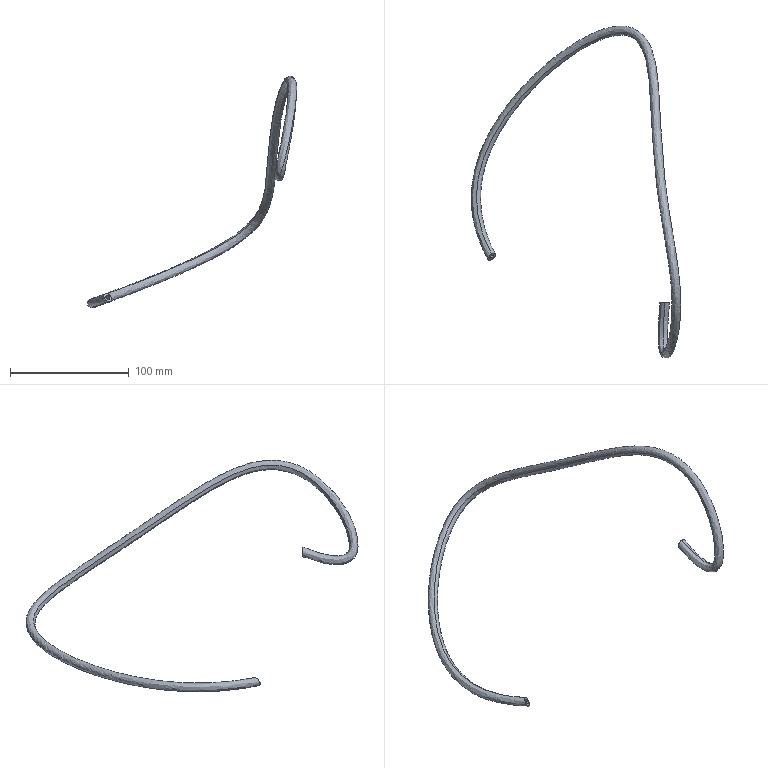Part | STEP file | 332_4 | 1 solid | 6 faces | box 176.185 x 279.344 x 194.737 mm | volume 23581 mm3 | spline 4 | plane 2